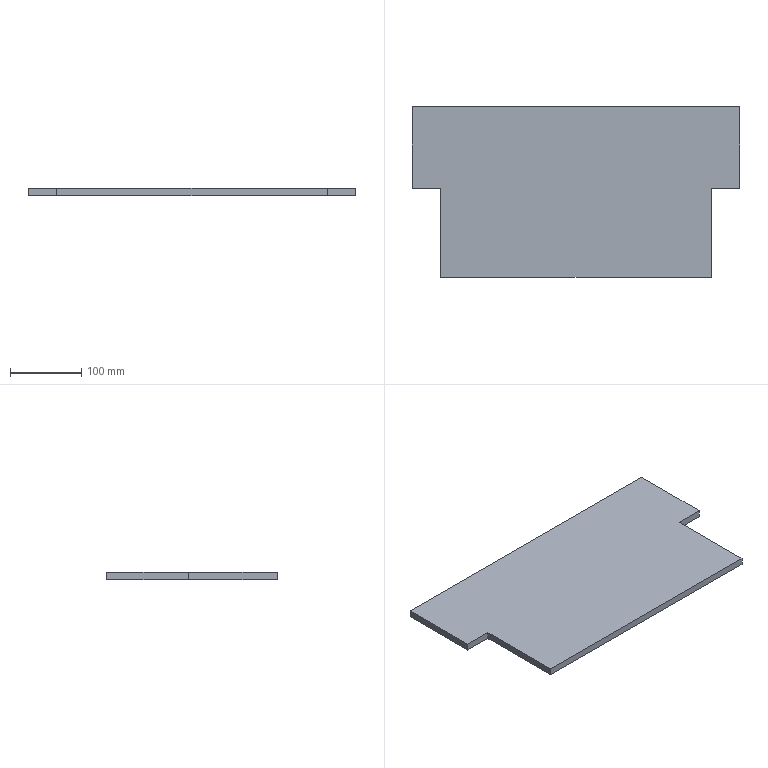Part | SolidWorks | features ICE 2, Extrusion 1 | 1 solid | 10 faces | box 460 x 240 x 10 mm | volume 1004000 mm3 | plane 10
STEP:
#1=CARTESIAN_POINT('',(0.,0.,0.));
#2=VERTEX_POINT('',#1);
#3=CARTESIAN_POINT('',(0.,-115.,0.));
#4=VERTEX_POINT('',#3);
#5=CARTESIAN_POINT('',(0.,0.,0.));
#6=DIRECTION('',(0.,-1.,0.));
#7=VECTOR('',#6,1000.);
#8=LINE('',#5,#7);
#9=EDGE_CURVE('',#2,#4,#8,.T.);
#10=ORIENTED_EDGE('',*,*,#9,.T.);
#11=CARTESIAN_POINT('',(0.,-115.,10.));
#12=VERTEX_POINT('',#11);
#13=CARTESIAN_POINT('',(0.,-115.,10.));
#14=DIRECTION('',(0.,0.,-1.));
#15=VECTOR('',#14,1000.);
#16=LINE('',#13,#15);
#17=EDGE_CURVE('',#12,#4,#16,.T.);
#18=ORIENTED_EDGE('',*,*,#17,.F.);
#19=CARTESIAN_POINT('',(0.,0.,10.));
#20=VERTEX_POINT('',#19);
#21=CARTESIAN_POINT('',(0.,0.,10.));
#22=DIRECTION('',(0.,-1.,0.));
#23=VECTOR('',#22,1000.);
#24=LINE('',#21,#23);
#25=EDGE_CURVE('',#20,#12,#24,.T.);
#26=ORIENTED_EDGE('',*,*,#25,.F.);
#27=CARTESIAN_POINT('',(0.,0.,10.));
#28=DIRECTION('',(0.,0.,-1.));
#29=VECTOR('',#28,1000.);
#30=LINE('',#27,#29);
#31=EDGE_CURVE('',#20,#2,#30,.T.);
#32=ORIENTED_EDGE('',*,*,#31,.T.);
#33=EDGE_LOOP('',(#10,#18,#26,#32));
#34=FACE_OUTER_BOUND('',#33,.T.);
#35=CARTESIAN_POINT('',(0.,0.,10.));
#36=DIRECTION('',(1.,0.,0.));
#37=DIRECTION('',(0.,1.,0.));
#38=AXIS2_PLACEMENT_3D('',#35,#36,#37);
#39=PLANE('',#38);
#40=ADVANCED_FACE('',(#34),#39,.F.);
#41=CARTESIAN_POINT('',(40.,-115.,0.));
#42=VERTEX_POINT('',#41);
#43=CARTESIAN_POINT('',(0.,-115.,0.));
#44=DIRECTION('',(1.,0.,0.));
#45=VECTOR('',#44,1000.);
#46=LINE('',#43,#45);
#47=EDGE_CURVE('',#4,#42,#46,.T.);
#48=ORIENTED_EDGE('',*,*,#47,.T.);
#49=CARTESIAN_POINT('',(40.,-115.,10.));
#50=VERTEX_POINT('',#49);
#51=CARTESIAN_POINT('',(40.,-115.,10.));
#52=DIRECTION('',(0.,0.,-1.));
#53=VECTOR('',#52,1000.);
#54=LINE('',#51,#53);
#55=EDGE_CURVE('',#50,#42,#54,.T.);
#56=ORIENTED_EDGE('',*,*,#55,.F.);
#57=CARTESIAN_POINT('',(0.,-115.,10.));
#58=DIRECTION('',(1.,0.,0.));
#59=VECTOR('',#58,1000.);
#60=LINE('',#57,#59);
#61=EDGE_CURVE('',#12,#50,#60,.T.);
#62=ORIENTED_EDGE('',*,*,#61,.F.);
#63=ORIENTED_EDGE('',*,*,#17,.T.);
#64=EDGE_LOOP('',(#48,#56,#62,#63));
#65=FACE_OUTER_BOUND('',#64,.T.);
#66=CARTESIAN_POINT('',(0.,-115.,10.));
#67=DIRECTION('',(0.,1.,0.));
#68=DIRECTION('',(0.,0.,1.));
#69=AXIS2_PLACEMENT_3D('',#66,#67,#68);
#70=PLANE('',#69);
#71=ADVANCED_FACE('',(#65),#70,.F.);
#72=CARTESIAN_POINT('',(40.,-240.,0.));
#73=VERTEX_POINT('',#72);
#74=CARTESIAN_POINT('',(420.,-240.,0.));
#75=VERTEX_POINT('',#74);
#76=CARTESIAN_POINT('',(410.,-240.,0.));
#77=DIRECTION('',(1.,0.,0.));
#78=VECTOR('',#77,1000.);
#79=LINE('',#76,#78);
#80=EDGE_CURVE('',#73,#75,#79,.T.);
#81=ORIENTED_EDGE('',*,*,#80,.T.);
#82=CARTESIAN_POINT('',(420.,-240.,10.));
#83=VERTEX_POINT('',#82);
#84=CARTESIAN_POINT('',(420.,-240.,10.));
#85=DIRECTION('',(0.,0.,-1.));
#86=VECTOR('',#85,1000.);
#87=LINE('',#84,#86);
#88=EDGE_CURVE('',#83,#75,#87,.T.);
#89=ORIENTED_EDGE('',*,*,#88,.F.);
#90=CARTESIAN_POINT('',(40.,-240.,10.));
#91=VERTEX_POINT('',#90);
#92=CARTESIAN_POINT('',(410.,-240.,10.));
#93=DIRECTION('',(1.,0.,0.));
#94=VECTOR('',#93,1000.);
#95=LINE('',#92,#94);
#96=EDGE_CURVE('',#91,#83,#95,.T.);
#97=ORIENTED_EDGE('',*,*,#96,.F.);
#98=CARTESIAN_POINT('',(40.,-240.,0.));
#99=DIRECTION('',(0.,0.,1.));
#100=VECTOR('',#99,1000.);
#101=LINE('',#98,#100);
#102=EDGE_CURVE('',#73,#91,#101,.T.);
#103=ORIENTED_EDGE('',*,*,#102,.F.);
#104=EDGE_LOOP('',(#81,#89,#97,#103));
#105=FACE_OUTER_BOUND('',#104,.T.);
#106=CARTESIAN_POINT('',(410.,-240.,10.));
#107=DIRECTION('',(0.,1.,0.));
#108=DIRECTION('',(0.,0.,1.));
#109=AXIS2_PLACEMENT_3D('',#106,#107,#108);
#110=PLANE('',#109);
#111=ADVANCED_FACE('',(#105),#110,.F.);
#112=CARTESIAN_POINT('',(420.,-115.,10.));
#113=VERTEX_POINT('',#112);
#114=CARTESIAN_POINT('',(460.,-115.,10.));
#115=VERTEX_POINT('',#114);
#116=CARTESIAN_POINT('',(460.,-115.,10.));
#117=DIRECTION('',(1.,0.,0.));
#118=VECTOR('',#117,1000.);
#119=LINE('',#116,#118);
#120=EDGE_CURVE('',#113,#115,#119,.T.);
#121=ORIENTED_EDGE('',*,*,#120,.F.);
#122=CARTESIAN_POINT('',(420.,-115.,0.));
#123=VERTEX_POINT('',#122);
#124=CARTESIAN_POINT('',(420.,-115.,0.));
#125=DIRECTION('',(0.,0.,1.));
#126=VECTOR('',#125,1000.);
#127=LINE('',#124,#126);
#128=EDGE_CURVE('',#123,#113,#127,.T.);
#129=ORIENTED_EDGE('',*,*,#128,.F.);
#130=CARTESIAN_POINT('',(460.,-115.,0.));
#131=VERTEX_POINT('',#130);
#132=CARTESIAN_POINT('',(460.,-115.,0.));
#133=DIRECTION('',(1.,0.,0.));
#134=VECTOR('',#133,1000.);
#135=LINE('',#132,#134);
#136=EDGE_CURVE('',#123,#131,#135,.T.);
#137=ORIENTED_EDGE('',*,*,#136,.T.);
#138=CARTESIAN_POINT('',(460.,-115.,10.));
#139=DIRECTION('',(0.,0.,-1.));
#140=VECTOR('',#139,1000.);
#141=LINE('',#138,#140);
#142=EDGE_CURVE('',#115,#131,#141,.T.);
#143=ORIENTED_EDGE('',*,*,#142,.F.);
#144=EDGE_LOOP('',(#121,#129,#137,#143));
#145=FACE_OUTER_BOUND('',#144,.T.);
#146=CARTESIAN_POINT('',(460.,-115.,10.));
#147=DIRECTION('',(0.,1.,0.));
#148=DIRECTION('',(0.,0.,1.));
#149=AXIS2_PLACEMENT_3D('',#146,#147,#148);
#150=PLANE('',#149);
#151=ADVANCED_FACE('',(#145),#150,.F.);
#152=CARTESIAN_POINT('',(460.,0.,0.));
#153=VERTEX_POINT('',#152);
#154=CARTESIAN_POINT('',(460.,0.,0.));
#155=DIRECTION('',(0.,1.,0.));
#156=VECTOR('',#155,1000.);
#157=LINE('',#154,#156);
#158=EDGE_CURVE('',#131,#153,#157,.T.);
#159=ORIENTED_EDGE('',*,*,#158,.T.);
#160=CARTESIAN_POINT('',(460.,0.,10.));
#161=VERTEX_POINT('',#160);
#162=CARTESIAN_POINT('',(460.,0.,10.));
#163=DIRECTION('',(0.,0.,-1.));
#164=VECTOR('',#163,1000.);
#165=LINE('',#162,#164);
#166=EDGE_CURVE('',#161,#153,#165,.T.);
#167=ORIENTED_EDGE('',*,*,#166,.F.);
#168=CARTESIAN_POINT('',(460.,0.,10.));
#169=DIRECTION('',(0.,1.,0.));
#170=VECTOR('',#169,1000.);
#171=LINE('',#168,#170);
#172=EDGE_CURVE('',#115,#161,#171,.T.);
#173=ORIENTED_EDGE('',*,*,#172,.F.);
#174=ORIENTED_EDGE('',*,*,#142,.T.);
#175=EDGE_LOOP('',(#159,#167,#173,#174));
#176=FACE_OUTER_BOUND('',#175,.T.);
#177=CARTESIAN_POINT('',(460.,0.,10.));
#178=DIRECTION('',(-1.,0.,0.));
#179=DIRECTION('',(0.,0.,1.));
#180=AXIS2_PLACEMENT_3D('',#177,#178,#179);
#181=PLANE('',#180);
#182=ADVANCED_FACE('',(#176),#181,.F.);
#183=CARTESIAN_POINT('',(0.,0.,0.));
#184=DIRECTION('',(-1.,0.,0.));
#185=VECTOR('',#184,1000.);
#186=LINE('',#183,#185);
#187=EDGE_CURVE('',#153,#2,#186,.T.);
#188=ORIENTED_EDGE('',*,*,#187,.T.);
#189=ORIENTED_EDGE('',*,*,#31,.F.);
#190=CARTESIAN_POINT('',(0.,0.,10.));
#191=DIRECTION('',(-1.,0.,0.));
#192=VECTOR('',#191,1000.);
#193=LINE('',#190,#192);
#194=EDGE_CURVE('',#161,#20,#193,.T.);
#195=ORIENTED_EDGE('',*,*,#194,.F.);
#196=ORIENTED_EDGE('',*,*,#166,.T.);
#197=EDGE_LOOP('',(#188,#189,#195,#196));
#198=FACE_OUTER_BOUND('',#197,.T.);
#199=CARTESIAN_POINT('',(0.,0.,10.));
#200=DIRECTION('',(0.,-1.,0.));
#201=DIRECTION('',(0.,0.,-1.));
#202=AXIS2_PLACEMENT_3D('',#199,#200,#201);
#203=PLANE('',#202);
#204=ADVANCED_FACE('',(#198),#203,.F.);
#205=CARTESIAN_POINT('',(420.,-115.,10.));
#206=DIRECTION('',(0.,-1.,0.));
#207=VECTOR('',#206,1000.);
#208=LINE('',#205,#207);
#209=EDGE_CURVE('',#113,#83,#208,.T.);
#210=ORIENTED_EDGE('',*,*,#209,.F.);
#211=ORIENTED_EDGE('',*,*,#120,.T.);
#212=ORIENTED_EDGE('',*,*,#172,.T.);
#213=ORIENTED_EDGE('',*,*,#194,.T.);
#214=ORIENTED_EDGE('',*,*,#25,.T.);
#215=ORIENTED_EDGE('',*,*,#61,.T.);
#216=CARTESIAN_POINT('',(40.,-240.,10.));
#217=DIRECTION('',(0.,1.,0.));
#218=VECTOR('',#217,1000.);
#219=LINE('',#216,#218);
#220=EDGE_CURVE('',#91,#50,#219,.T.);
#221=ORIENTED_EDGE('',*,*,#220,.F.);
#222=ORIENTED_EDGE('',*,*,#96,.T.);
#223=EDGE_LOOP('',(#210,#211,#212,#213,#214,#215,#221,#222));
#224=FACE_OUTER_BOUND('',#223,.T.);
#225=CARTESIAN_POINT('',(0.,0.,10.));
#226=DIRECTION('',(0.,0.,1.));
#227=DIRECTION('',(1.,0.,0.));
#228=AXIS2_PLACEMENT_3D('',#225,#226,#227);
#229=PLANE('',#228);
#230=ADVANCED_FACE('',(#224),#229,.T.);
#231=ORIENTED_EDGE('',*,*,#136,.F.);
#232=CARTESIAN_POINT('',(420.,-240.,0.));
#233=DIRECTION('',(0.,1.,0.));
#234=VECTOR('',#233,1000.);
#235=LINE('',#232,#234);
#236=EDGE_CURVE('',#75,#123,#235,.T.);
#237=ORIENTED_EDGE('',*,*,#236,.F.);
#238=ORIENTED_EDGE('',*,*,#80,.F.);
#239=CARTESIAN_POINT('',(40.,-115.,0.));
#240=DIRECTION('',(0.,-1.,0.));
#241=VECTOR('',#240,1000.);
#242=LINE('',#239,#241);
#243=EDGE_CURVE('',#42,#73,#242,.T.);
#244=ORIENTED_EDGE('',*,*,#243,.F.);
#245=ORIENTED_EDGE('',*,*,#47,.F.);
#246=ORIENTED_EDGE('',*,*,#9,.F.);
#247=ORIENTED_EDGE('',*,*,#187,.F.);
#248=ORIENTED_EDGE('',*,*,#158,.F.);
#249=EDGE_LOOP('',(#231,#237,#238,#244,#245,#246,#247,#248));
#250=FACE_OUTER_BOUND('',#249,.T.);
#251=CARTESIAN_POINT('',(0.,0.,0.));
#252=DIRECTION('',(0.,0.,1.));
#253=DIRECTION('',(1.,0.,0.));
#254=AXIS2_PLACEMENT_3D('',#251,#252,#253);
#255=PLANE('',#254);
#256=ADVANCED_FACE('',(#250),#255,.F.);
#257=ORIENTED_EDGE('',*,*,#88,.T.);
#258=ORIENTED_EDGE('',*,*,#236,.T.);
#259=ORIENTED_EDGE('',*,*,#128,.T.);
#260=ORIENTED_EDGE('',*,*,#209,.T.);
#261=EDGE_LOOP('',(#257,#258,#259,#260));
#262=FACE_OUTER_BOUND('',#261,.T.);
#263=CARTESIAN_POINT('',(420.,0.,0.));
#264=DIRECTION('',(1.,0.,0.));
#265=DIRECTION('',(0.,0.,-1.));
#266=AXIS2_PLACEMENT_3D('',#263,#264,#265);
#267=PLANE('',#266);
#268=ADVANCED_FACE('',(#262),#267,.T.);
#269=ORIENTED_EDGE('',*,*,#55,.T.);
#270=ORIENTED_EDGE('',*,*,#243,.T.);
#271=ORIENTED_EDGE('',*,*,#102,.T.);
#272=ORIENTED_EDGE('',*,*,#220,.T.);
#273=EDGE_LOOP('',(#269,#270,#271,#272));
#274=FACE_OUTER_BOUND('',#273,.T.);
#275=CARTESIAN_POINT('',(40.,0.,0.));
#276=DIRECTION('',(-1.,0.,0.));
#277=DIRECTION('',(0.,0.,1.));
#278=AXIS2_PLACEMENT_3D('',#275,#276,#277);
#279=PLANE('',#278);
#280=ADVANCED_FACE('',(#274),#279,.T.);
#281=CLOSED_SHELL('',(#40,#71,#111,#151,#182,#204,#230,#256,#268,#280));
#282=MANIFOLD_SOLID_BREP('',#281);
#283=CARTESIAN_POINT('',(0.,0.,0.));
#284=DIRECTION('',(0.,0.,1.));
#285=DIRECTION('',(1.,0.,0.));
#286=AXIS2_PLACEMENT_3D('',#283,#284,#285);
#287=(LENGTH_UNIT()NAMED_UNIT(*)SI_UNIT(.MILLI.,.METRE.));
#288=UNCERTAINTY_MEASURE_WITH_UNIT(LENGTH_MEASURE(0.00001),#287,'','');
#289=(NAMED_UNIT(*)PLANE_ANGLE_UNIT()SI_UNIT($,.RADIAN.));
#290=(NAMED_UNIT(*)SI_UNIT($,.STERADIAN.)SOLID_ANGLE_UNIT());
#291=(GEOMETRIC_REPRESENTATION_CONTEXT(3)GLOBAL_UNCERTAINTY_ASSIGNED_CONTEXT((#288))GLOBAL_UNIT_ASSIGNED_CONTEXT((#287,#289,#290))REPRESENTATION_CONTEXT('',''));
#292=ADVANCED_BREP_SHAPE_REPRESENTATION('',(#282,#286),#291);